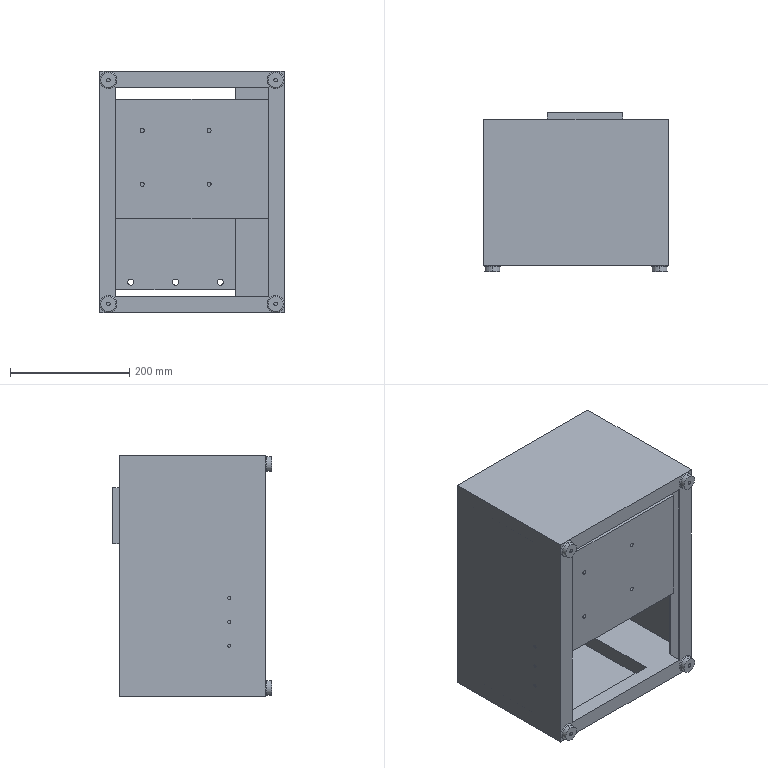Part | SolidWorks | features BaseBody 7, MoveFace 3, Split 2, CombineBodies 1, DelFace 1, ICE 1, MoveCopyBody 1 | 1 solid | 160 faces | box 309 x 266.4 x 404 mm | volume 2740160 mm3 | plane 102 | cylinder 50 | torus 8 | commonest cylinder face diameters 10.5 x12 6 x8 6.8 x8 10.2 x8 25 x8 5 x6